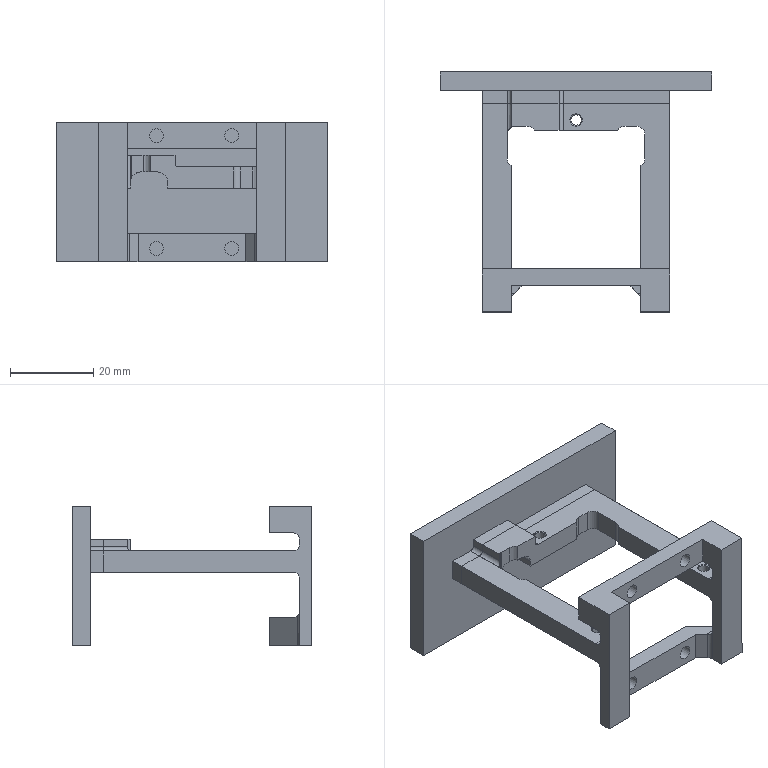NC program | NX | posted with a generic post | part box 65 x 57.5 x 33.5 mm
Whole program, first 1596 of 1898 lines:
N10 G17 G21 G94 G90
(PLANAR_MILL , TOOL : D50面刀)
N12 T01 M6
N14 G53
N16 G17 G0 G90 X52.5 Y-0.5 B0. C0. S3500 M3
N18 G43 Z30.05 H1
N20 Z2.05
N22 G94 G1 Z0.05 F1000.
N24 X25.5
N26 X-25.5
N28 X-52.5
N30 Z2.05
N32 G0 Z30.05
N34 M5
(动态粗 , TOOL : D8-25-D8-60-3T-ROUGH)
N36 T02 M6
N38 G53
N40 G17 G0 G90 X-0.557 Y27.041 B0. C0. S6500 M3
N42 G43 Z30.2 H2
N44 Z-19.5
N46 G94 G1 X-0.555 Y27.016 Z-19.656 F3000.
N48 X-0.553 Y26.991 Z-19.718
N50 X-0.551 Y26.966 Z-19.763
N52 X-0.549 Y26.941 Z-19.8
N54 X-0.548 Y26.916 Z-19.831
N56 X-0.546 Y26.891 Z-19.857
N58 X-0.544 Y26.866 Z-19.88
N60 X-0.542 Y26.841 Z-19.9
N62 X-0.54 Y26.816 Z-19.918
N64 X-0.538 Y26.792 Z-19.933
N66 X-0.536 Y26.767 Z-19.947
N68 X-0.534 Y26.742 Z-19.958
N70 X-0.532 Y26.717 Z-19.968
N72 X-0.53 Y26.692 Z-19.977
N74 X-0.528 Y26.667 Z-19.984
N76 X-0.526 Y26.642 Z-19.99
N78 X-0.525 Y26.617 Z-19.994
N80 X-0.523 Y26.592 Z-19.997
N82 X-0.521 Y26.567 Z-19.999
N84 X-0.519 Y26.542 Z-20.
N86 X-0.415 Y25.2
N88 G3 X0.016 Y24.546 R0.809
N90 X2.614 Y23.818 R7.174
N92 X8.686 Y23.525 R57.315
N94 G1 X23.204 Y23.487
N96 G2 X26.087 Y21.863 R4.371
N98 X27.84 Y18.076 R8.759
N100 X28.414 Y12.488 R30.165
N102 X28.496 Y0.339 R489.81
N104 G1 Y-18.003
N106 G2 X26.977 Y-20.994 R4.21
N108 X23.16 Y-22.822 R8.565
N110 X17.5 Y-23.414 R29.674
N112 X5.276 Y-23.496 R488.293
N114 G1 X-23.021
N116 G2 X-26.01 Y-21.973 R4.208
N118 X-27.81 Y-18.22 R8.513
N120 X-28.405 Y-12.786 R28.448
N122 X-28.496 Y-0.262 R446.293
N124 G1 X-28.495 Y18.022
N126 G2 X-27.03 Y20.961 R4.192
N128 X-23.299 Y22.793 R8.358
N130 X-17.792 Y23.405 R28.015
N132 X-2.672 Y23.477 R466.577
N134 X1.584 Y22.966 R87.011
N136 G3 X10.708 Y22.525 R86.358
N138 G1 X20.58 Y22.488
N140 G2 X24.717 Y20.326 R5.87
N142 X26.404 Y18.298 R4.575
N144 X27.231 Y13.537 R21.682
N146 X27.484 Y4.692 R121.912
N148 G1 X27.495 Y-3.858
N150 X27.485 Y-15.603
N152 G2 X25.908 Y-19.17 R5.72
N154 G1 X25.784 Y-19.369
N156 G2 X23.693 Y-20.871 R5.631
N158 X18.624 Y-22.148 R16.146
N160 X11.284 Y-22.469 R76.065
N162 G1 X1.235 Y-22.496
N164 X-20.471 Y-22.492
N166 G2 X-24.743 Y-20.301 R5.816
N168 X-25.789 Y-19.372 R5.228
N170 X-26.624 Y-17.58 R4.87
N172 X-27.37 Y-11.259 R33.14
N174 X-27.495 Y1.639 R373.69
N176 G1 X-27.496 Y15.322
N178 G2 X-25.942 Y19.135 R5.618
N180 X-24.013 Y20.719 R4.745
N182 X-19.05 Y22.098 R14.951
N184 X-11.938 Y22.462 R64.82
N186 X-3.839 Y22.452 R189.088
N188 X2.452 Y21.889 R227.028
N190 G3 X13.92 Y21.514 R149.911
N192 G2 X18.783 Y21.465 R106.716
N194 X20.893 Y20.966 R8.221
N196 G1 X22.579 Y20.95
N198 G2 X25.558 Y19.628 R4.379
N200 X26.7 Y16.749 R4.363
N202 G1 Y-16.751
N204 X26.595 Y-17.685
N206 X26.284 Y-18.572
N208 X25.784 Y-19.369
N210 X25.119 Y-20.034
N212 X24.322 Y-20.534
N214 X23.435 Y-20.845
N216 G2 X21.599 Y-20.95 R8.97
N218 X7.654 Y-21.481 R161.576
N220 G1 X-1.346 Y-21.495
N222 X-18.92 Y-21.488
N224 G2 X-20.949 Y-20.969 R8.256
N226 G3 X-22.587 Y-20.95 R17.96
N228 G2 X-24.364 Y-20.519 R4.885
N230 G1 X-24.87 Y-20.197
N232 X-24.364 Y-20.519
N234 G3 X-22.587 Y-20.95 R4.887
N236 G1 X21.671
N238 G2 X22.255 Y-22.297 R0.8
N240 X21.801 Y-22.553 Z-19.966 R1.018
N242 G1 X20.825 Y-22.902 Z-19.9
N244 X19.451 Y-23.393 F15000.
N246 X19.318 Y-23.426
N248 X19.182 Y-23.439
N250 X-24.367
N252 G2 X-26.65 Y-22.283 R2.833
N254 G1 X-27.499 Y-21.126
N256 G2 X-27.558 Y-20.265 R0.83
N258 G1 X-26.941 Y-18.827 Z-20. F3000.
N260 X-26.77 Y-18.436
N262 G3 X-26.588 Y-17.726 R1.479
N264 G1 X-26.7 Y-16.782
N266 Y16.751
N268 G2 X-25.557 Y19.63 R4.366
N270 X-22.578 Y20.95 R4.377
N272 G3 X-19.164 Y21.126 R31.383
N274 G2 X-4.473 Y21.421 R151.648
N276 X1.766 Y20.95 R256.713
N278 G1 X21.041
N280 G3 X21.328 Y22.497 R0.8
N282 G1 X19.817 Y22.903 Z-19.9
N284 X19.394 Y23.018 F15000.
N286 X18.967 Y23.121
N288 X18.863 Y23.128
N290 X3.945
N292 G3 X3.408 Y22.921 R0.806
N294 G1 X3.277 Y22.767 Z-19.913 F3000.
N296 X3.174 Y22.593 Z-19.926
N298 X2.596 Y21.588 Z-20.
N300 X2.393 Y21.252
N302 G2 X1.766 Y20.95 R0.802
N304 G1 X-21.634
N306 G2 X-22.431 Y21.626 R0.808
N308 G1 X-22.642 Y22.902
N310 X-22.646 Y22.927 Z-19.999
N312 X-22.65 Y22.951 Z-19.997
N314 X-22.654 Y22.976 Z-19.994
N316 X-22.658 Y23.001 Z-19.99
N318 X-22.662 Y23.025 Z-19.984
N320 X-22.666 Y23.05 Z-19.977
N322 X-22.671 Y23.075 Z-19.968
N324 X-22.675 Y23.099 Z-19.958
N326 X-22.679 Y23.124 Z-19.947
N328 X-22.683 Y23.149 Z-19.933
N330 X-22.687 Y23.173 Z-19.918
N332 X-22.691 Y23.198 Z-19.9
N334 X-22.695 Y23.223 Z-19.88
N336 X-22.699 Y23.247 Z-19.857
N338 X-22.703 Y23.272 Z-19.831
N340 X-22.707 Y23.297 Z-19.8
N342 X-22.711 Y23.321 Z-19.763
N344 X-22.715 Y23.346 Z-19.718
N346 X-22.72 Y23.371 Z-19.656
N348 X-22.724 Y23.395 Z-19.5
N350 G0 Z30.2
N352 X-3.658 Y-3.32
N354 Z0.5
N356 G3 X-3.658 Y-3.32 Z0.105 I-1.698 J3.174
N358 X-3.658 Y-3.32 Z-0.29 I-1.698 J3.174
N360 X-3.658 Y-3.32 Z-0.684 I-1.698 J3.174
N362 X-3.658 Y-3.32 Z-1.079 I-1.698 J3.174
N364 X-3.658 Y-3.32 Z-1.474 I-1.698 J3.174
N366 X-3.658 Y-3.32 Z-1.869 I-1.698 J3.174
N368 X-3.658 Y-3.32 Z-2.264 I-1.698 J3.174
N370 X-3.658 Y-3.32 Z-2.659 I-1.698 J3.174
N372 X-3.658 Y-3.32 Z-3.053 I-1.698 J3.174
N374 X-3.658 Y-3.32 Z-3.448 I-1.698 J3.174
N376 X-3.658 Y-3.32 Z-3.843 I-1.698 J3.174
N378 X-3.658 Y-3.32 Z-4.238 I-1.698 J3.174
N380 X-3.658 Y-3.32 Z-4.633 I-1.698 J3.174
N382 X-3.658 Y-3.32 Z-5.028 I-1.698 J3.174
N384 X-3.658 Y-3.32 Z-5.422 I-1.698 J3.174
N386 X-3.658 Y-3.32 Z-5.817 I-1.698 J3.174
N388 X-3.658 Y-3.32 Z-6.212 I-1.698 J3.174
N390 X-3.658 Y-3.32 Z-6.607 I-1.698 J3.174
N392 X-3.658 Y-3.32 Z-7.002 I-1.698 J3.174
N394 X-3.658 Y-3.32 Z-7.396 I-1.698 J3.174
N396 X-3.658 Y-3.32 Z-7.791 I-1.698 J3.174
N398 X-3.658 Y-3.32 Z-8.186 I-1.698 J3.174
N400 X-3.658 Y-3.32 Z-8.581 I-1.698 J3.174
N402 X-3.658 Y-3.32 Z-8.976 I-1.698 J3.174
N404 X-3.658 Y-3.32 Z-9.371 I-1.698 J3.174
N406 X-3.658 Y-3.32 Z-9.765 I-1.698 J3.174
N408 X-3.658 Y-3.32 Z-10.16 I-1.698 J3.174
N410 X-3.658 Y-3.32 Z-10.555 I-1.698 J3.174
N412 X-3.658 Y-3.32 Z-10.95 I-1.698 J3.174
N414 X-3.658 Y-3.32 Z-11.345 I-1.698 J3.174
N416 X-3.658 Y-3.32 Z-11.74 I-1.698 J3.174
N418 X-3.658 Y-3.32 Z-12.134 I-1.698 J3.174
N420 X-3.658 Y-3.32 Z-12.529 I-1.698 J3.174
N422 X-3.658 Y-3.32 Z-12.924 I-1.698 J3.174
N424 X-3.658 Y-3.32 Z-13.319 I-1.698 J3.174
N426 X-3.658 Y-3.32 Z-13.714 I-1.698 J3.174
N428 X-3.658 Y-3.32 Z-14.108 I-1.698 J3.174
N430 X-3.658 Y-3.32 Z-14.503 I-1.698 J3.174
N432 X-3.658 Y-3.32 Z-14.898 I-1.698 J3.174
N434 X-3.658 Y-3.32 Z-15.293 I-1.698 J3.174
N436 X-3.658 Y-3.32 Z-15.688 I-1.698 J3.174
N438 X-3.658 Y-3.32 Z-16.083 I-1.698 J3.174
N440 X-3.658 Y-3.32 Z-16.477 I-1.698 J3.174
N442 X-3.658 Y-3.32 Z-16.872 I-1.698 J3.174
N444 X-3.658 Y-3.32 Z-17.267 I-1.698 J3.174
N446 X-3.658 Y-3.32 Z-17.662 I-1.698 J3.174
N448 X-3.658 Y-3.32 Z-18.057 I-1.698 J3.174
N450 X-3.658 Y-3.32 Z-18.452 I-1.698 J3.174
N452 X-3.658 Y-3.32 Z-18.846 I-1.698 J3.174
N454 X-3.658 Y-3.32 Z-19.241 I-1.698 J3.174
N456 X-3.658 Y-3.32 Z-19.636 I-1.698 J3.174
N458 X-5.356 Y-3.746 Z-20. R-3.6
N460 X-8.859 Y0.86 R-3.622
N462 X-7.565 Y-3.074 R3.686
N464 X-1.257 Y-0.404 R3.803
N466 X-8.737 Y-2.568 R-4.133
N468 X-0.763 Y0.472 R4.371
N470 X-9.596 Y-2.153 R-4.663
N472 X-0.197 Y0.395 R4.928
N474 X-10.258 Y-2.033 R-5.22
N476 X0.396 Y0.253 R5.501
N478 X-11.072 Y-1.317 R-5.8
N480 X-8.712 Y-5.051 R6.09
N482 X-6.404 Y-6.109 R5.892
N484 X-4.011 Y-6.078 R25.458
N486 X1.014 Y-0.352 R5.969
N488 X-2.88 Y5.767 R6.345
N490 G1 X-3.058 Y5.8
N492 X-7.004 Y5.79
N494 G3 X-10.686 Y3.432 R5.323
N496 X-11.295 Y2.231 R3.646
N498 G1 X-11.287 Y-1.937
N500 G3 X-9.152 Y-5.489 R5.512
N502 X-8.184 Y-6.084 R3.454
N504 X-6.386 Y-6.109 R15.894
N506 G1 X-8.261 Y-6.105
N508 G2 X-10.345 Y-4.765 R3.942
N510 X-11.289 Y-3.176 R4.436
N512 G1 X-11.3 Y-1.745
N514 X-11.285 Y-3.669
N516 G3 X-9.606 Y-6.046 R3.591
N518 G1 X-9.335 Y-6.109
N520 X-8.135
N522 X-9.56 Y-6.104
N524 G2 X-11.28 Y-4.463 R2.722
N526 X-11.3 Y-3.507 R14.66
N528 G1 X-11.283 Y-4.769
N530 G3 X-10.436 Y-6.026 R1.868
N532 G1 X-10.128 Y-6.109
N534 X-9.453
N536 G2 X-10.452 Y-6.069 R3.999
N538 X-11.3 Y-5.07 R1.309
N540 G1 Y-4.62
N542 G3 X-11.26 Y-5.459 R3.698
N544 X-10.162 Y-6.109 R0.982
N546 G1 X-2.885 Y-6.096
N548 G3 X0.214 Y-4.217 R4.93
N550 X-1.467 Y5.723 R6.84
N552 G1 X-1.76 Y5.8
N554 X-3.11
N556 X-1.61
N558 G2 X0.114 Y4.765 R3.423
N560 X-0.224 Y-5.193 R6.955
N562 X-1.699 Y-6.091 R4.625
N564 X-3.096 Y-6.109 R24.229
N566 G3 X-1.183 Y-6.077 R16.279
N568 X1.17 Y-4.492 R4.334
N570 X0.54 Y5.228 R7.352
N572 X-0.308 Y5.785 R1.994
N574 G1 X-1.685 Y5.8
N576 X-0.185 Y5.794
N578 G2 X1.544 Y4.545 R3.475
N580 X1.363 Y-4.834 R7.503
N582 X-0.323 Y-6.086 R4.306
N584 X-1.521 Y-6.109 R8.553
N586 G3 X0.057 Y-6.087 R16.365
N588 X2.198 Y-4.634 R3.913
N590 X3.49 Y2.138 R7.698
N592 X1.312 Y5.621 R6.406
N594 X0.833 Y5.8 R1.065
N596 G1 X-0.292
N598 X1.057 Y5.795
N600 G2 X2.618 Y4.671 R3.155
N602 X4.144 Y-0.576 R7.5
N604 X2.037 Y-5.335 R7.228
N606 X0.86 Y-6.094 R3.079
N608 G1 X-0.143 Y-6.109
N610 G3 X1.339 Y-6.066 R8.535
N612 X3.42 Y-4.506 R4.035
N614 X4.562 Y2.281 R8.024
N616 X2.594 Y5.553 R6.327
N618 X2.032 Y5.8 R1.021
N620 G1 X0.982
N622 X2.257 Y5.794
N624 G2 X3.81 Y4.624 R3.109
N626 X5.241 Y-0.438 R7.624
N628 X3.293 Y-5.214 R7.44
N630 X2.051 Y-6.083 R3.529
N632 X1.004 Y-6.109 R5.719
N634 G3 X2.35 Y-6.091 R35.512
N636 X4.329 Y-4.758 R3.592
N638 X5.926 Y0.73 R7.853
N640 X4.199 Y5.131 R7.317
N642 X3.328 Y5.779 R1.966
N644 X2.14 Y5.8 R11.657
N646 G1 X3.414 Y5.795
N648 G2 X4.878 Y4.712 R2.954
N650 X6.352 Y0.036 R7.493
N652 X4.55 Y-5.06 R7.745
N654 X3.176 Y-6.084 R3.544
N656 X2.203 Y-6.109 R5.878
N658 G3 X3.483 Y-6.088 R17.141
N660 X5.459 Y-4.722 R3.575
N662 X7.029 Y0.74 R7.949
N664 X5.422 Y5.035 R7.397
N666 X4.527 Y5.764 R2.287
N668 X3.289 Y5.8 R6.426
N670 G1 X4.563 Y5.794
N672 G2 X6.084 Y4.615 R3.027
N674 X7.451 Y-0.121 R7.618
N676 X5.659 Y-5.055 R7.762
N678 X4.323 Y-6.073 R3.885
N680 X3.309 Y-6.109 R4.91
N682 G3 X4.587 Y-6.089 R20.116
N684 X6.558 Y-4.725 R3.565
N686 X8.138 Y0.69 R7.989
N688 X6.578 Y5.003 R7.442
N690 X5.695 Y5.754 R2.464
N692 G1 X5.475 Y5.8
N694 X4.425
N696 X5.625
N698 G2 X6.94 Y4.94 R2.475
N700 X8.514 Y1.023 R6.976
N702 X7.035 Y-4.724 R8.249
N704 X5.401 Y-6.08 R3.963
N706 X4.417 Y-6.109 R4.438
N708 G1 X5.668 Y-6.094
N710 G3 X7.529 Y-4.886 R3.434
N712 X9.257 Y0.013 R7.786
N714 X7.835 Y4.833 R7.755
N716 X6.847 Y5.743 R2.918
N718 G1 X6.597 Y5.8
N720 X5.622
N722 X6.747
N724 G2 X8.063 Y4.936 R2.474
N726 X9.632 Y0.922 R7.01
N728 X8.109 Y-4.76 R8.227
N730 X6.55 Y-6.068 R4.257
N732 X5.513 Y-6.109 R4.583
N734 G1 X6.782 Y-6.091
N736 G3 X8.668 Y-4.838 R3.448
N738 X10.365 Y0.118 R7.857
N740 X8.918 Y4.877 R7.69
N742 X8.005 Y5.727 R3.189
N744 G1 X7.715 Y5.8
N746 X6.74
N748 X7.865
N750 G2 X9.167 Y4.95 R2.457
N752 X10.732 Y0.977 R6.956
N754 X9.148 Y-4.84 R8.209
N756 X7.667 Y-6.063 R4.243
N758 X6.622 Y-6.109 R4.195
N760 G3 X7.895 Y-6.09 R28.393
N762 X9.864 Y-4.726 R3.566
N764 X11.3 Y-1.485 R7.324
N766 X11.273 Y1.564 R49.051
N768 X9.521 Y5.421 R6.195
N770 X8.817 Y5.8 R1.157
N772 G1 X7.842
N774 X9.042 Y5.794
N776 G2 X10.557 Y4.573 R2.98
N778 X11.3 Y3.024 R4.23
N780 G1 Y1.149
N782 X11.285 Y3.699
N784 G3 X10.104 Y5.693 R3.046
N786 X9.747 Y5.8 R2.866
N788 G1 X8.922
N790 X9.897
N792 G2 X11.111 Y4.838 R1.973
N794 X11.3 Y4.338 R1.246
N796 G1 Y3.513
N798 G3 X11.279 Y4.776 R13.612
N800 X10.572 Y5.743 R1.302
N802 X9.874 Y5.8 R1.848
N804 G2 X10.72 Y5.733 R2.207
N806 X11.3 Y4.587 R1.09
N808 G3 X11.097 Y5.47 R1.263
N810 X10.678 Y5.749 R1.014
N812 G2 X11.271 Y5.11 R0.873
N814 G1 X11.3 Y4.887
N816 X11.287 Y-2.268
N818 G2 X8.862 Y-6.017 R5.053
N820 G1 X8.531 Y-6.109
N822 X7.706
N824 X8.961 Y-6.093
N826 G3 X10.866 Y-4.758 R3.351
N828 X11.3 Y-3.911 R1.768
N830 G1 Y-2.036
N832 Y-4.061
N834 G2 X9.646 Y-6.085 R2.734
N836 X8.823 Y-6.109 R6.586
N838 G3 X9.953 Y-6.085 R8.9
N840 X11.238 Y-5.122 R1.964
N842 G1 X11.3 Y-4.856
N844 Y-4.031
N846 Y-5.006
N848 G2 X10.21 Y-6.109 R1.37
N850 G1 X9.76
N852 G3 X10.65 Y-6.069 R3.988
N854 X11.3 Y-4.971 R0.982
N856 X10.857 Y-4.207 R0.881
N858 G1 X10.699 Y-4.117
N860 X9.341 Y-3.34 Z-19.9
N862 X-3.211 Y3.834 F15000.
N864 X-4.569 Y4.611 Z-20. F3000.
N866 X-6.446 Y5.684
N868 G3 X-6.883 Y5.8 R0.9
N870 X-8.373 Y5.744 R7.486
N872 X-11.235 Y3.628 R4.771
N874 G1 X-11.3 Y3.35
N876 Y2.15
N878 Y3.5
N880 G2 X-10.238 Y5.121 R2.944
N882 X-9.087 Y5.791 R2.934
N884 G1 X-7.962 Y5.8
N886 X-9.514 Y5.784
N888 G3 X-11.21 Y4.655 R2.676
N890 G1 X-11.3 Y4.328
N892 Y3.428
N894 Y4.478
N896 G2 X-10.03 Y5.794 R1.78
N898 G1 X-9.376 Y5.8
N900 G3 X-10.412 Y5.774 R6.347
N902 X-11.287 Y4.967 R1.112
N904 G1 X-11.3 Y4.427
N906 G2 X-11.179 Y5.344 R1.826
N908 X-10.237 Y5.8 R0.951
N910 G3 X-10.818 Y5.695 R1.166
N912 X-11.222 Y5.248 R0.862
N914 X-10.68 Y4.179 R0.808
N916 G1 X-9.337 Y3.813
N918 X-9.313 Y3.806 Z-19.999
N920 X-9.289 Y3.8 Z-19.997
N922 X-9.264 Y3.793 Z-19.994
N924 X-9.24 Y3.786 Z-19.99
N926 X-9.216 Y3.78 Z-19.984
N928 X-9.192 Y3.773 Z-19.977
N930 X-9.168 Y3.767 Z-19.968
N932 X-9.144 Y3.76 Z-19.958
N934 X-9.12 Y3.754 Z-19.947
N936 X-9.096 Y3.747 Z-19.933
N938 X-9.071 Y3.74 Z-19.918
N940 X-9.047 Y3.734 Z-19.9
N942 X-9.023 Y3.727 Z-19.88
N944 X-8.999 Y3.721 Z-19.857
N946 X-8.975 Y3.714 Z-19.831
N948 X-8.951 Y3.708 Z-19.8
N950 X-8.927 Y3.701 Z-19.763
N952 X-8.903 Y3.694 Z-19.718
N954 X-8.879 Y3.688 Z-19.656
N956 X-8.854 Y3.681 Z-19.5
N958 G0 Z30.2
N960 X-13.615 Y23.401
N962 Z-5.7
N964 G1 X-13.612 Y23.376 Z-5.856
N966 X-13.608 Y23.352 Z-5.918
N968 X-13.605 Y23.327 Z-5.964
N970 X-13.602 Y23.302 Z-6.
N972 X-13.598 Y23.277 Z-6.031
N974 X-13.595 Y23.252 Z-6.057
N976 X-13.591 Y23.228 Z-6.08
N978 X-13.588 Y23.203 Z-6.1
N980 X-13.585 Y23.178 Z-6.118
N982 X-13.581 Y23.153 Z-6.133
N984 X-13.578 Y23.129 Z-6.147
N986 X-13.574 Y23.104 Z-6.158
N988 X-13.571 Y23.079 Z-6.168
N990 X-13.568 Y23.054 Z-6.177
N992 X-13.564 Y23.03 Z-6.184
N994 X-13.561 Y23.005 Z-6.19
N996 X-13.557 Y22.98 Z-6.194
N998 X-13.554 Y22.955 Z-6.198
N1000 X-13.55 Y22.93 Z-6.199
N1002 X-13.547 Y22.906 Z-6.2
N1004 X-13.368 Y21.604
N1006 G3 X-12.654 Y20.91 R0.808
N1008 G1 X-12.082 Y20.849
N1010 G3 X-8.705 Y20.163 R11.109
N1012 X-1.005 Y19.957 R110.469
N1014 G1 X10.087 Y19.953
N1016 X10.39 Y20.045
N1018 X11.188 Y20.541
N1020 X12.082 Y20.849
N1022 X12.678 Y20.913
N1024 X12.082 Y20.849
N1026 X11.188 Y20.541
N1028 G2 X10.151 Y19.916 R9.659
N1030 X7.314 Y19.475 R10.662
N1032 X-3.84 Y19.387 R192.319
N1034 X-9.65 Y19.731 R45.951
N1036 X-10.386 Y20.042 R1.126
N1038 G3 X-11.259 Y20.565 R36.07
N1040 G2 X-10.31 Y19.968 R5.604
N1042 G3 X-8.885 Y19.171 R3.052
N1044 X-4.648 Y18.528 R18.337
N1046 X6.951 Y18.511 R109.452
N1048 X9.24 Y18.878 R10.047
N1050 X9.714 Y19.377 R1.13
N1052 G1 X10.386 Y20.042
N1054 X9.714 Y19.377
N1056 G2 X8.809 Y18.585 R1.478
N1058 X5.568 Y17.954 R11.199
N1060 X-5.804 Y18.066 R74.975
N1062 X-9.21 Y18.841 R11.936
N1064 X-9.714 Y19.377 R1.174
N1066 G1 X-10.14 Y19.799
N1068 G2 X-9.392 Y18.87 R3.109
N1070 G3 X-7.597 Y17.793 R4.089
N1072 X-3.244 Y17.016 R17.771
N1074 X5.796 Y17.063 R52.282
N1076 X8.732 Y17.815 R8.817
N1078 X9.207 Y18.579 R1.274
N1080 G1 X9.529 Y19.086
N1082 G3 X9.024 Y18.064 R2.816
N1084 G2 X8.082 Y17.31 R2.072
N1086 X4.654 Y16.484 R10.658
N1088 X-5.322 Y16.723 R41.444
N1090 X-8.53 Y17.761 R9.708
N1092 X-9.207 Y18.579 R1.195
N1094 G1 X-9.408 Y18.896
N1096 G2 X-9.033 Y18.088 R2.481
N1098 G3 X-7.659 Y16.842 R3.111
N1100 X-3.706 Y15.697 R12.047
N1102 X5.307 Y15.686 R32.782
N1104 X8.359 Y16.714 R8.073
N1106 X8.891 Y17.689 R1.081
N1108 G1 X9.067 Y18.183
N1110 G3 X8.834 Y17.209 R2.524
N1112 G2 X8.034 Y16.292 R1.818
N1114 X4.861 Y15.177 R8.286
N1116 X-5.073 Y15.428 R28.131
N1118 X-8.232 Y16.751 R8.571
N1120 X-8.858 Y17.485 R1.501
N1122 G3 X-9.041 Y18.113 R2.699
N1124 G2 X-8.849 Y17.335 R2.106
N1126 G3 X-7.842 Y16.004 R2.568
N1128 X-4.331 Y14.514 R9.107
N1130 X5.189 Y14.387 R23.99
N1132 X8.189 Y15.629 R7.632
N1134 X8.78 Y16.488 R1.23
N1136 G2 X8.85 Y17.347 R7.238
N1138 G3 X8.774 Y16.263 R7.612
N1140 G2 X7.766 Y15.057 R2.443
N1142 X4.428 Y13.798 R8.7
N1144 X-5.093 Y14.209 R21.894
N1146 X-8.217 Y15.853 R7.677
N1148 X-8.78 Y16.713 R1.624
N1150 G1 X-8.85 Y17.345
N1152 X-8.755 Y16.35
N1154 G3 X-7.539 Y14.744 R3.252
N1156 X-4.273 Y13.28 R7.788
N1158 X5.422 Y13.194 R18.849
N1160 X8.307 Y14.688 R7.014
N1162 X8.78 Y15.473 R1.249
N1164 G1 Y16.373
N1166 Y15.323
N1168 G2 X7.888 Y14.042 R2.375
N1170 G1 X7.139 Y13.485
N1172 G3 X6.624 Y11.079 R2.764
N1174 X8.469 Y8.225 R5.262
N1176 X10.067 Y7.003 R67.019
N1178 X10.776 Y6.376 R14.395
N1180 G2 X11.3 Y5.517 R1.435
N1182 G1 Y5.142
N1184 G3 X11.125 Y6.117 R1.636
N1186 X10.183 Y6.875 R4.64
N1188 G2 X8.874 Y9.125 R4.537
N1190 G1 X8.78 Y10.001
N1192 Y15.326
N1194 G3 X8.366 Y16.072 R0.881
N1196 X7.814 Y16.215 Z-6.163 R1.09
N1198 G1 X6.829 Y16.287 Z-6.1
N1200 X-6.87 Y17.294 F15000.
N1202 X-7.412 Y17.338 Z-6.135 F3000.
N1204 X-7.955 Y17.366 Z-6.17
N1206 G3 X-8.4 Y17.212 Z-6.2 R0.917
N1208 X-8.78 Y16.488 R0.881
N1210 X-8.125 Y14.722 R2.388
N1212 X-6.701 Y13.517 R6.523
N1214 G2 X-6.229 Y11.901 R2.24
N1216 X-7.506 Y9.352 R3.792
N1218 X-9.278 Y7.97 R14.227
N1220 G3 X-9.591 Y7.527 R1.783
N1222 G2 X-10.843 Y6.4 R4.753
N1224 G3 X-11.3 Y5.554 R1.057
N1226 G1 Y5.179
N1228 X-11.292 Y5.668
N1230 G2 X-10.948 Y6.312 R1.006
N1232 G1 X-10.183 Y6.875
N1234 X-9.591 Y7.527
N1236 G3 X-8.835 Y8.806 R23.849
N1238 X-8.536 Y12.34 R6.037
N1240 G1 X-8.78 Y13.522
N1242 Y16.147
N1244 Y9.999
N1246 G2 X-9.149 Y8.288 R4.873
N1248 G1 X-9.337 Y7.964
N1250 G3 X-9.214 Y6.99 R0.808
N1252 G1 X-8.289 Y6.052
N1254 X-8.272 Y6.034 Z-6.199
N1256 X-8.254 Y6.016 Z-6.198
N1258 X-8.236 Y5.998 Z-6.194
N1260 X-8.219 Y5.981 Z-6.19
N1262 X-8.201 Y5.963 Z-6.184
N1264 X-8.184 Y5.945 Z-6.177
N1266 X-8.166 Y5.927 Z-6.168
N1268 X-8.149 Y5.909 Z-6.158
N1270 X-8.131 Y5.892 Z-6.147
N1272 X-8.114 Y5.874 Z-6.133
N1274 X-8.096 Y5.856 Z-6.118
N1276 X-8.078 Y5.838 Z-6.1
N1278 X-8.061 Y5.82 Z-6.08
N1280 X-8.043 Y5.803 Z-6.057
N1282 X-8.026 Y5.785 Z-6.031
N1284 X-8.008 Y5.767 Z-6.
N1286 X-7.991 Y5.749 Z-5.964
N1288 X-7.973 Y5.731 Z-5.918
N1290 X-7.956 Y5.714 Z-5.856
N1292 X-7.938 Y5.696 Z-5.7
N1294 G0 Z30.2
N1296 X-13.137 Y23.389
N1298 Z-5.5
N1300 G1 X-13.132 Y23.364 Z-5.656
N1302 X-13.128 Y23.34 Z-5.718
N1304 X-13.124 Y23.315 Z-5.763
N1306 X-13.119 Y23.29 Z-5.8
N1308 X-13.115 Y23.266 Z-5.831
N1310 X-13.111 Y23.241 Z-5.857
N1312 X-13.106 Y23.216 Z-5.88
N1314 X-13.102 Y23.192 Z-5.9
N1316 X-13.097 Y23.167 Z-5.918
N1318 X-13.093 Y23.143 Z-5.933
N1320 X-13.089 Y23.118 Z-5.947
N1322 X-13.084 Y23.093 Z-5.958
N1324 X-13.08 Y23.069 Z-5.968
N1326 X-13.076 Y23.044 Z-5.977
N1328 X-13.071 Y23.02 Z-5.984
N1330 X-13.067 Y22.995 Z-5.99
N1332 X-13.062 Y22.97 Z-5.994
N1334 X-13.058 Y22.946 Z-5.997
N1336 X-13.054 Y22.921 Z-5.999
N1338 X-13.049 Y22.897 Z-6.
N1340 X-12.794 Y21.462
N1342 G3 X-12.264 Y20.84 R0.809
N1344 G1 X-11.385 Y20.534
N1346 X-10.584 Y20.035
N1348 X-9.914 Y19.371
N1350 X-9.406 Y18.575
N1352 X-9.087 Y17.687
N1354 X-8.973 Y16.749
N1356 Y9.999
N1358 G2 X-9.721 Y7.62 R4.534
N1360 X-10.879 Y6.5 R4.764
N1362 G3 X-11.232 Y6.018 R1.139
N1364 X-10.362 Y4.921 R0.808
N1366 G1 X-9.338 Y5.073
N1368 X-9.313 Y5.077 Z-5.999
N1370 X-9.288 Y5.081 Z-5.997
N1372 X-9.264 Y5.084 Z-5.994
N1374 X-9.239 Y5.088 Z-5.99
N1376 X-9.214 Y5.092 Z-5.984
N1378 X-9.189 Y5.095 Z-5.977
N1380 X-9.165 Y5.099 Z-5.968
N1382 X-9.14 Y5.103 Z-5.958
N1384 X-9.115 Y5.106 Z-5.947
N1386 X-9.09 Y5.11 Z-5.933
N1388 X-9.066 Y5.114 Z-5.918
N1390 X-9.041 Y5.117 Z-5.9
N1392 X-9.016 Y5.121 Z-5.88
N1394 X-8.992 Y5.125 Z-5.857
N1396 X-8.967 Y5.128 Z-5.831
N1398 X-8.942 Y5.132 Z-5.8
N1400 X-8.917 Y5.136 Z-5.763
N1402 X-8.893 Y5.139 Z-5.718
N1404 X-8.868 Y5.143 Z-5.656
N1406 X-8.843 Y5.147 Z-5.5
N1408 G0 Z30.2
N1410 X-14.832 Y23.401
N1412 Z-4.5
N1414 G1 X-14.828 Y23.376 Z-4.656
N1416 X-14.824 Y23.351 Z-4.718
N1418 X-14.821 Y23.326 Z-4.763
N1420 X-14.817 Y23.302 Z-4.8
N1422 X-14.814 Y23.277 Z-4.831
N1424 X-14.81 Y23.252 Z-4.857
N1426 X-14.807 Y23.227 Z-4.88
N1428 X-14.803 Y23.203 Z-4.9
N1430 X-14.8 Y23.178 Z-4.918
N1432 X-14.796 Y23.153 Z-4.933
N1434 X-14.793 Y23.128 Z-4.947
N1436 X-14.789 Y23.104 Z-4.958
N1438 X-14.785 Y23.079 Z-4.968
N1440 X-14.782 Y23.054 Z-4.977
N1442 X-14.778 Y23.029 Z-4.984
N1444 X-14.775 Y23.005 Z-4.99
N1446 X-14.771 Y22.98 Z-4.994
N1448 X-14.768 Y22.955 Z-4.997
N1450 X-14.764 Y22.93 Z-4.999
N1452 X-14.761 Y22.906 Z-5.
N1454 X-14.573 Y21.598
N1456 G3 X-13.866 Y20.91 R0.808
N1458 G1 X-13.278 Y20.842
N1460 X-12.388 Y20.53
N1462 X-11.589 Y20.03
N1464 X-10.919 Y19.367
N1466 X-10.411 Y18.572
N1468 X-10.09 Y17.685
N1470 X-9.973 Y16.749
N1472 Y9.999
N1474 G2 X-11.064 Y7.19 R4.338
N1476 G3 X-11.3 Y6.536 R1.111
N1478 G1 Y5.936
N1480 G3 X-10.496 Y5.128 R0.808
N1482 G1 X-9.331 Y5.122
N1484 X-9.306 Z-4.999
N1486 X-9.281 Z-4.997
N1488 X-9.256 Z-4.994
N1490 X-9.231 Z-4.99
N1492 X-9.206 Z-4.984
N1494 X-9.181 Z-4.977
N1496 X-9.156 Z-4.968
N1498 X-9.131 Z-4.958
N1500 X-9.106 Y5.121 Z-4.947
N1502 X-9.081 Z-4.933
N1504 X-9.056 Z-4.918
N1506 X-9.031 Z-4.9
N1508 X-9.006 Z-4.88
N1510 X-8.981 Z-4.857
N1512 X-8.956 Z-4.831
N1514 X-8.931 Z-4.8
N1516 X-8.906 Z-4.763
N1518 X-8.881 Y5.12 Z-4.718
N1520 X-8.856 Z-4.656
N1522 X-8.831 Z-4.5
N1524 G0 Z30.2
N1526 X-15.783 Y23.401
N1528 Z-3.5
N1530 G1 X-15.78 Y23.376 Z-3.656
N1532 X-15.776 Y23.352 Z-3.718
N1534 X-15.773 Y23.327 Z-3.763
N1536 X-15.77 Y23.302 Z-3.8
N1538 X-15.766 Y23.277 Z-3.831
N1540 X-15.763 Y23.252 Z-3.857
N1542 X-15.759 Y23.228 Z-3.88
N1544 X-15.756 Y23.203 Z-3.9
N1546 X-15.752 Y23.178 Z-3.918
N1548 X-15.749 Y23.153 Z-3.933
N1550 X-15.746 Y23.129 Z-3.947
N1552 X-15.742 Y23.104 Z-3.958
N1554 X-15.739 Y23.079 Z-3.968
N1556 X-15.735 Y23.054 Z-3.977
N1558 X-15.732 Y23.03 Z-3.984
N1560 X-15.729 Y23.005 Z-3.99
N1562 X-15.725 Y22.98 Z-3.994
N1564 X-15.722 Y22.955 Z-3.997
N1566 X-15.718 Y22.93 Z-3.999
N1568 X-15.715 Y22.906 Z-4.
N1570 X-15.535 Y21.603
N1572 G3 X-14.824 Y20.91 R0.808
N1574 G1 X-14.244 Y20.846
N1576 X-13.354 Y20.536
N1578 X-12.556 Y20.036
N1580 X-11.888 Y19.371
N1582 X-11.386 Y18.575
N1584 X-11.073 Y17.686
N1586 X-10.966 Y16.749
N1588 Y9.938
N1590 G2 X-11.283 Y8.273 R5.42
N1592 G1 X-11.3 Y6.744
N1594 G3 X-10.366 Y5.946 R0.808
N1596 G1 X-9.341 Y6.108
N1598 X-9.316 Y6.112 Z-3.999
N1600 X-9.291 Y6.115 Z-3.997
N1602 X-9.266 Y6.119 Z-3.994
N1604 X-9.242 Y6.123 Z-3.99
N1606 X-9.217 Y6.127 Z-3.984
N1608 X-9.192 Y6.131 Z-3.977
N1610 X-9.168 Y6.135 Z-3.968
N1612 X-9.143 Y6.139 Z-3.958
N1614 X-9.118 Y6.143 Z-3.947
N1616 X-9.094 Y6.147 Z-3.933
N1618 X-9.069 Y6.151 Z-3.918
N1620 X-9.044 Y6.154 Z-3.9
N1622 X-9.02 Y6.158 Z-3.88
N1624 X-8.995 Y6.162 Z-3.857
N1626 X-8.97 Y6.166 Z-3.831
N1628 X-8.945 Y6.17 Z-3.8
N1630 X-8.921 Y6.174 Z-3.763
N1632 X-8.896 Y6.178 Z-3.718
N1634 X-8.871 Y6.182 Z-3.656
N1636 X-8.847 Y6.186 Z-3.5
N1638 G0 Z30.2
N1640 X-15.883 Y23.403
N1642 Z-2.5
N1644 G1 X-15.88 Y23.378 Z-2.656
N1646 X-15.878 Y23.353 Z-2.718
N1648 X-15.875 Y23.328 Z-2.763
N1650 X-15.872 Y23.303 Z-2.8
N1652 X-15.869 Y23.279 Z-2.831
N1654 X-15.867 Y23.254 Z-2.857
N1656 X-15.864 Y23.229 Z-2.88
N1658 X-15.861 Y23.204 Z-2.9
N1660 X-15.859 Y23.179 Z-2.918
N1662 X-15.856 Y23.154 Z-2.933
N1664 X-15.853 Y23.129 Z-2.947
N1666 X-15.851 Y23.105 Z-2.958
N1668 X-15.848 Y23.08 Z-2.968
N1670 X-15.845 Y23.055 Z-2.977
N1672 X-15.843 Y23.03 Z-2.984
N1674 X-15.84 Y23.005 Z-2.99
N1676 X-15.837 Y22.98 Z-2.994
N1678 X-15.834 Y22.955 Z-2.997
N1680 X-15.832 Y22.931 Z-2.999
N1682 X-15.829 Y22.906 Z-3.
N1684 X-15.689 Y21.614
N1686 G3 X-14.966 Y20.897 R0.808
N1688 G1 X-14.653 Y20.866
N1690 X-13.842 Y20.609
N1692 X-13.022 Y20.141
N1694 X-12.328 Y19.503
N1696 X-11.794 Y18.725
N1698 G2 X-11.331 Y17.295 R5.639
N1700 G1 X-11.3 Y16.736
N1702 Y8.261
N1704 G3 X-10.601 Y7.46 R0.808
N1706 G1 X-9.344 Y7.288
N1708 X-9.319 Y7.285 Z-2.999
N1710 X-9.295 Y7.282 Z-2.997
N1712 X-9.27 Y7.278 Z-2.994
N1714 X-9.245 Y7.275 Z-2.99
N1716 X-9.22 Y7.272 Z-2.984
N1718 X-9.196 Y7.268 Z-2.977
N1720 X-9.171 Y7.265 Z-2.968
N1722 X-9.146 Y7.261 Z-2.958
N1724 X-9.121 Y7.258 Z-2.947
N1726 X-9.097 Y7.255 Z-2.933
N1728 X-9.072 Y7.251 Z-2.918
N1730 X-9.047 Y7.248 Z-2.9
N1732 X-9.022 Y7.244 Z-2.88
N1734 X-8.997 Y7.241 Z-2.857
N1736 X-8.973 Y7.238 Z-2.831
N1738 X-8.948 Y7.234 Z-2.8
N1740 X-8.923 Y7.231 Z-2.763
N1742 X-8.898 Y7.228 Z-2.718
N1744 X-8.874 Y7.224 Z-2.656
N1746 X-8.849 Y7.221 Z-2.5
N1748 G0 Z30.2
N1750 X8.849 Y4.682
N1752 Z-5.5
N1754 G1 X8.874 Y4.685 Z-5.656
N1756 X8.899 Y4.689 Z-5.718
N1758 X8.923 Y4.692 Z-5.763
N1760 X8.948 Y4.696 Z-5.8
N1762 X8.973 Y4.699 Z-5.831
N1764 X8.998 Y4.703 Z-5.857
N1766 X9.022 Y4.707 Z-5.88
N1768 X9.047 Y4.71 Z-5.9
N1770 X9.072 Y4.714 Z-5.918
N1772 X9.097 Y4.717 Z-5.933
N1774 X9.121 Y4.721 Z-5.947
N1776 X9.146 Y4.724 Z-5.958
N1778 X9.171 Y4.728 Z-5.968
N1780 X9.196 Y4.731 Z-5.977
N1782 X9.22 Y4.735 Z-5.984
N1784 X9.245 Y4.738 Z-5.99
N1786 X9.27 Y4.742 Z-5.994
N1788 X9.295 Y4.745 Z-5.997
N1790 X9.319 Y4.749 Z-5.999
N1792 X9.344 Y4.753 Z-6.
N1794 X10.591 Y4.931
N1796 G3 X11.227 Y6.029 R0.808
N1798 X10.877 Y6.5 R1.156
N1800 G2 X9.313 Y8.36 R4.477
N1802 X8.973 Y10.001 R4.892
N1804 G1 Y16.751
N1806 X9.093 Y17.708
N1808 X9.426 Y18.614
N1810 X9.955 Y19.422
N1812 X10.652 Y20.089
N1814 X11.483 Y20.581
N1816 X12.34 Y20.854
N1818 G3 X12.891 Y21.481 R0.809
N1820 G1 X13.146 Y22.894
N1822 X13.15 Y22.918 Z-5.999
N1824 X13.154 Y22.943 Z-5.997
N1826 X13.159 Y22.968 Z-5.994
N1828 X13.163 Y22.992 Z-5.99
N1830 X13.168 Y23.017 Z-5.984
N1832 X13.172 Y23.041 Z-5.977
N1834 X13.177 Y23.066 Z-5.968
N1836 X13.181 Y23.091 Z-5.958
N1838 X13.185 Y23.115 Z-5.947
N1840 X13.19 Y23.14 Z-5.933
N1842 X13.194 Y23.164 Z-5.918
N1844 X13.199 Y23.189 Z-5.9
N1846 X13.203 Y23.214 Z-5.88
N1848 X13.208 Y23.238 Z-5.857
N1850 X13.212 Y23.263 Z-5.831
N1852 X13.216 Y23.287 Z-5.8
N1854 X13.221 Y23.312 Z-5.763
N1856 X13.225 Y23.337 Z-5.718
N1858 X13.23 Y23.361 Z-5.656
N1860 X13.234 Y23.386 Z-5.5
N1862 G0 Z30.2
N1864 X8.844 Y5.148
N1866 Z-4.5
N1868 G1 X8.869 Z-4.656
N1870 X8.894 Z-4.718
N1872 X8.919 Y5.149 Z-4.763
N1874 X8.944 Z-4.8
N1876 X8.969 Z-4.831
N1878 X8.994 Y5.15 Z-4.857
N1880 X9.019 Z-4.88
N1882 X9.044 Z-4.9
N1884 X9.069 Y5.151 Z-4.918
N1886 X9.094 Z-4.933
N1888 X9.119 Z-4.947
N1890 X9.144 Y5.152 Z-4.958
N1892 X9.169 Z-4.968
N1894 X9.194 Z-4.977
N1896 X9.219 Y5.153 Z-4.984
N1898 X9.244 Z-4.99
N1900 X9.269 Z-4.994
N1902 X9.294 Y5.154 Z-4.997
N1904 X9.319 Z-4.999
N1906 X9.344 Z-5.
N1908 X10.503 Y5.17
N1910 G3 X11.3 Y5.97 R0.808
N1912 X11.031 Y6.805 R2.959
N1914 X10.731 Y7.626 R6.4
N1916 G2 X9.973 Y10.001 R4.292
N1918 G1 Y16.751
N1920 X10.083 Y17.689
N1922 X10.4 Y18.579
N1924 X10.907 Y19.377
N1926 X11.578 Y20.042
N1928 X12.381 Y20.541
N1930 X13.274 Y20.848
N1932 X13.871 Y20.913
N1934 X13.274 Y20.848
N1936 X12.381 Y20.541
N1938 X11.578 Y20.042
N1940 X10.907 Y19.377
N1942 X10.4 Y18.579
N1944 X10.083 Y17.689
N1946 X9.973 Y16.751
N1948 Y10.001
N1950 G3 X11.063 Y7.191 R4.338
N1952 G2 X11.3 Y6.538 R1.109
N1954 G1 Y5.938
N1956 G2 X10.496 Y5.13 R0.808
N1958 G1 X9.344 Y5.124
N1960 X9.319 Z-4.999
N1962 X9.294 Y5.123 Z-4.997
N1964 X9.269 Z-4.994
N1966 X9.244 Z-4.99
N1968 X9.219 Z-4.984
N1970 X9.194 Z-4.977
N1972 X9.169 Z-4.968
N1974 X9.144 Z-4.958
N1976 X9.119 Y5.122 Z-4.947
N1978 X9.094 Z-4.933
N1980 X9.069 Z-4.918
N1982 X9.044 Z-4.9
N1984 X9.019 Z-4.88
N1986 X8.994 Z-4.857
N1988 X8.969 Z-4.831
N1990 X8.944 Y5.121 Z-4.8
N1992 X8.919 Z-4.763
N1994 X8.894 Z-4.718
N1996 X8.869 Z-4.656
N1998 X8.844 Z-4.5
N2000 G0 Z30.2
N2002 X8.83 Y6.278
N2004 Z-3.5
N2006 G1 X8.855 Y6.275 Z-3.656
N2008 X8.88 Y6.271 Z-3.718
N2010 X8.904 Y6.267 Z-3.763
N2012 X8.929 Y6.263 Z-3.8
N2014 X8.954 Y6.259 Z-3.831
N2016 X8.978 Y6.255 Z-3.857
N2018 X9.003 Y6.251 Z-3.88
N2020 X9.028 Y6.247 Z-3.9
N2022 X9.052 Y6.243 Z-3.918
N2024 X9.077 Y6.239 Z-3.933
N2026 X9.102 Y6.235 Z-3.947
N2028 X9.126 Y6.231 Z-3.958
N2030 X9.151 Y6.227 Z-3.968
N2032 X9.176 Y6.223 Z-3.977
N2034 X9.2 Y6.219 Z-3.984
N2036 X9.225 Y6.215 Z-3.99
N2038 X9.25 Y6.211 Z-3.994
N2040 X9.275 Y6.207 Z-3.997
N2042 X9.299 Y6.203 Z-3.999
N2044 X9.324 Y6.199 Z-4.
N2046 X10.351 Y6.035
N2048 G3 X11.286 Y6.833 R0.808
N2050 G1 X11.119 Y8.858
N2052 G2 X10.966 Y9.934 R3.906
N2054 G1 Y16.75
N2056 X11.068 Y17.688
N2058 X11.378 Y18.58
N2060 X11.88 Y19.379
N2062 X12.548 Y20.045
N2064 X13.348 Y20.544
N2066 X14.24 Y20.851
N2068 X14.837 Y20.914
N2070 X14.24 Y20.851
N2072 X13.348 Y20.544
N2074 X12.548 Y20.045
N2076 X11.88 Y19.379
N2078 X11.378 Y18.58
N2080 X11.068 Y17.688
N2082 X10.966 Y16.75
N2084 Y9.934
N2086 G3 X11.252 Y8.398 R4.579
N2088 G2 X11.286 Y6.884 R10.327
N2090 X10.351 Y6.086 R0.808
N2092 G1 X9.324 Y6.25
N2094 X9.299 Y6.254 Z-3.999
N2096 X9.274 Y6.258 Z-3.997
N2098 X9.25 Y6.262 Z-3.994
N2100 X9.225 Y6.266 Z-3.99
N2102 X9.2 Y6.27 Z-3.984
N2104 X9.176 Y6.274 Z-3.977
N2106 X9.151 Y6.278 Z-3.968
N2108 X9.126 Y6.282 Z-3.958
N2110 X9.102 Y6.286 Z-3.947
N2112 X9.077 Y6.29 Z-3.933
N2114 X9.052 Y6.294 Z-3.918
N2116 X9.028 Y6.298 Z-3.9
N2118 X9.003 Y6.302 Z-3.88
N2120 X8.978 Y6.305 Z-3.857
N2122 X8.954 Y6.309 Z-3.831
N2124 X8.929 Y6.313 Z-3.8
N2126 X8.904 Y6.317 Z-3.763
N2128 X8.879 Y6.321 Z-3.718
N2130 X8.855 Y6.325 Z-3.656
N2132 X8.83 Y6.329 Z-3.5
N2134 G0 Z30.2
N2136 X8.849 Y7.298
N2138 Z-2.5
N2140 G1 X8.874 Y7.301 Z-2.656
N2142 X8.898 Y7.305 Z-2.718
N2144 X8.923 Y7.308 Z-2.763
N2146 X8.948 Y7.311 Z-2.8
N2148 X8.973 Y7.315 Z-2.831
N2150 X8.997 Y7.318 Z-2.857
N2152 X9.022 Y7.321 Z-2.88
N2154 X9.047 Y7.325 Z-2.9
N2156 X9.072 Y7.328 Z-2.918
N2158 X9.097 Y7.332 Z-2.933
N2160 X9.121 Y7.335 Z-2.947
N2162 X9.146 Y7.338 Z-2.958
N2164 X9.171 Y7.342 Z-2.968
N2166 X9.196 Y7.345 Z-2.977
N2168 X9.22 Y7.349 Z-2.984
N2170 X9.245 Y7.352 Z-2.99
N2172 X9.27 Y7.355 Z-2.994
N2174 X9.295 Y7.359 Z-2.997
N2176 X9.319 Y7.362 Z-2.999
N2178 X9.344 Y7.365 Z-3.
N2180 X10.601 Y7.537
N2182 G3 X11.3 Y8.338 R0.808
N2184 G1 Y16.752
N2186 G2 X11.697 Y18.533 R4.884
N2188 X12.812 Y19.977 R4.887
N2190 X14.826 Y20.893 R4.342
N2192 G3 X15.452 Y21.556 R0.809
N2194 G1 X15.665 Y22.896
N2196 X15.669 Y22.92 Z-2.999
N2198 X15.673 Y22.945 Z-2.997
N2200 X15.677 Y22.97 Z-2.994
N2202 X15.68 Y22.995 Z-2.99
N2204 X15.684 Y23.019 Z-2.984
N2206 X15.688 Y23.044 Z-2.977
N2208 X15.692 Y23.069 Z-2.968
N2210 X15.696 Y23.093 Z-2.958
N2212 X15.7 Y23.118 Z-2.947
N2214 X15.704 Y23.143 Z-2.933
N2216 X15.708 Y23.167 Z-2.918
N2218 X15.712 Y23.192 Z-2.9
N2220 X15.716 Y23.217 Z-2.88
N2222 X15.72 Y23.241 Z-2.857
N2224 X15.724 Y23.266 Z-2.831
N2226 X15.728 Y23.291 Z-2.8
N2228 X15.731 Y23.315 Z-2.763
N2230 X15.735 Y23.34 Z-2.718
N2232 X15.739 Y23.365 Z-2.656
N2234 X15.743 Y23.39 Z-2.5
N2236 G0 Z30.2
N2238 X-8.884 Y-3.751
N2240 Z-5.7
N2242 G1 X-8.907 Y-3.761 Z-5.856
N2244 X-8.93 Y-3.771 Z-5.918
N2246 X-8.953 Y-3.781 Z-5.964
N2248 X-8.976 Y-3.79 Z-6.
N2250 X-8.999 Y-3.8 Z-6.031
N2252 X-9.022 Y-3.81 Z-6.057
N2254 X-9.045 Y-3.819 Z-6.08
N2256 X-9.068 Y-3.829 Z-6.1
N2258 X-9.091 Y-3.839 Z-6.118
N2260 X-9.114 Y-3.849 Z-6.133
N2262 X-9.137 Y-3.858 Z-6.147
N2264 X-9.16 Y-3.868 Z-6.158
N2266 X-9.183 Y-3.878 Z-6.168
N2268 X-9.206 Y-3.888 Z-6.177
N2270 X-9.229 Y-3.897 Z-6.184
N2272 X-9.252 Y-3.907 Z-6.19
N2274 X-9.275 Y-3.917 Z-6.194
N2276 X-9.298 Y-3.926 Z-6.198
N2278 X-9.321 Y-3.936 Z-6.199
N2280 X-9.344 Y-3.946 Z-6.2
N2282 X-10.806 Y-4.563
N2284 G3 X-11.3 Y-5.307 R0.809
N2286 X-10.763 Y-6.212 R0.838
N2288 X-8.168 Y-6.826 R8.28
N2290 X-1.304 Y-7.091 R73.232
N2292 X8.941 Y-7.082 R385.152
N2294 X10.871 Y-6.526 R3.645
N2296 X11.3 Y-5.825 R0.921
N2298 G1 Y-5.3
N2300 X11.293 Y-6.049
N2302 G2 X10.448 Y-6.952 R1.556
N2304 X8.114 Y-7.51 R6.527
N2306 X1.747 Y-7.696 R75.555
N2308 X-6.873 Y-7.5 R118.833
N2310 X-10.195 Y-6.871 R11.926
N2312 X-11.19 Y-6.148 R2.038
N2314 X-11.3 Y-5.412 R1.312
N2316 G3 X-11.223 Y-6.288 R2.206
N2318 X-9.875 Y-7.444 R2.758
N2320 X-6.205 Y-8.352 R11.934
N2322 X1.827 Y-8.675 R75.442
N2324 X7.792 Y-8.447 R51.422
N2326 X10.544 Y-7.589 R6.669
N2328 X11.251 Y-6.856 R1.64
N2330 X11.3 Y-5.882 R3.568
N2332 G1 Y-6.782
N2334 G2 X10.594 Y-7.778 R1.706
N2336 X8.042 Y-8.807 R6.156
N2338 X2.785 Y-9.234 R30.966
N2340 X-5.926 Y-8.932 R69.036
N2342 X-9.742 Y-7.959 R12.287
N2344 X-11.216 Y-6.745 R3.392
N2346 X-11.3 Y-5.982 R1.76
N2348 G3 X-11.238 Y-6.941 R3.011
N2350 X-9.888 Y-8.408 R3.187
N2352 X-6.286 Y-9.663 R10.369
N2354 X0.802 Y-10.198 R43.066
N2356 X7.09 Y-9.854 R38.265
N2358 X10.352 Y-8.716 R8.397
N2360 X11.244 Y-7.815 R2.318
N2362 G1 X11.3 Y-7.569
N2364 Y-6.669
N2366 Y-7.719
N2368 G2 X10.499 Y-8.879 R2.102
N2370 X7.434 Y-10.22 R7.371
N2372 X1.678 Y-10.753 R28.661
N2374 X-6.109 Y-10.227 R41.409
N2376 X-9.891 Y-8.875 R10.748
N2378 X-11.239 Y-7.503 R3.724
N2380 X-11.3 Y-6.64 R2.571
N2382 G3 X-11.272 Y-7.693 R6.142
N2384 X-9.955 Y-9.41 R3.337
N2386 X-6.268 Y-10.974 R10.043
N2388 X0.943 Y-11.686 R33.394
N2390 X7.238 Y-11.13 R27.69
N2392 X10.555 Y-9.651 R8.201
N2394 X11.25 Y-8.842 R2.233
N2396 G1 X11.3 Y-8.616
N2398 Y-7.716
N2400 Y-8.766
N2402 G2 X10.396 Y-10.076 R2.431
N2404 X7.06 Y-11.614 R8.239
N2406 X0.683 Y-12.228 R26.695
N2408 X-6.42 Y-11.458 R30.215
N2410 X-10.096 Y-9.796 R9.978
N2412 X-11.259 Y-8.417 R3.774
N2414 X-11.3 Y-7.528 R3.765
N2416 G3 X-11.249 Y-8.777 R5.443
N2418 X-9.826 Y-10.628 R3.877
N2420 X-5.849 Y-12.393 R10.838
N2422 X6.051 Y-12.709 R30.577
N2424 X10.089 Y-11.159 R10.626
N2426 X11.224 Y-10.03 R3.75
N2428 G1 X11.3 Y-9.737
N2430 Y-8.762
N2432 X11.293 Y-9.962
N2434 G2 X10.17 Y-11.445 R3.077
N2436 X6.426 Y-13.093 R9.625
N2438 X-1.438 Y-13.588 R27.155
N2440 X-7.515 Y-12.388 R21.296
N2442 X-10.685 Y-10.349 R8.063
N2444 X-11.288 Y-9.363 R2.472
N2446 G1 X-11.3 Y-8.454
N2448 X-11.284 Y-9.709
N2450 G3 X-10.054 Y-11.61 R3.676
N2452 X-6.828 Y-13.388 R8.575
N2454 X-6.372 Y-13.322 R1.28
N2456 X-5.995 Y-12.008 Z-6.1 R0.883
N2458 G1 X-6.075 Y-11.909 F15000.
N2460 X-6.17 Y-11.822
N2462 X-9.335 Y-9.316
N2464 X-9.652 Y-9.061 Z-6.126 F3000.
N2466 X-9.977 Y-8.818 Z-6.152
N2468 G3 X-10.703 Y-8.745 Z-6.2 R0.893
N2470 X-11.3 Y-9.579 R0.88
N2472 X-10.552 Y-11.756 R2.907
N2474 X-8.844 Y-13.23 R7.316
N2476 G2 X-8.37 Y-14.846 R2.245
N2478 X-9.866 Y-17.592 R3.797
N2480 X-11.713 Y-18.73 R10.606
N2482 G3 X-12.457 Y-19.644 R6.985
N2484 G2 X-14.655 Y-20.864 R4.526
N2486 X-16.101 Y-20.95 R8.703
N2488 G3 X-13.844 Y-20.61 R5.292
N2490 X-11.887 Y-18.877 R4.421
N2492 X-10.771 Y-15.09 R4.952
N2494 X-11.296 Y-12.522 R15.753
N2496 G1 X-11.3 Y-10.08
N2498 Y-17.05
N2500 G2 X-11.9 Y-18.902 R4.196
N2502 G3 X-10.459 Y-19.597 R-0.8
N2504 G1 X-10.123 Y-18.84
N2506 X-9.616 Y-17.714 Z-6.121
N2508 X-9.523 Y-17.579 Z-6.111
N2510 X-9.406 Y-17.464 Z-6.1
N2512 X-9.232 Y-17.361 F15000.
N2514 X8.254 Y-9.873
N2516 X9.328 Y-9.471
N2518 X10.278 Y-9.121 Z-6.165 F3000.
N2520 G2 X10.817 Y-9.153 Z-6.2 R0.802
N2522 X11.3 Y-9.887 R0.801
N2524 X10.686 Y-11.286 R2.127
N2526 X7.703 Y-13.162 R7.157
N2528 G3 X6.925 Y-13.881 R1.297
N2530 X7.432 Y-17.732 R3.454
N2532 X10.402 Y-19.549 R6.469
N2534 X12.893 Y-20.079 R17.085
N2536 G2 X13.733 Y-20.56 R9.572
N2538 G1 X14.595 Y-20.851
N2540 X15.192 Y-20.916
N2542 X14.595 Y-20.851
N2544 G2 X12.656 Y-19.861 R4.934
N2546 X11.632 Y-19.12 R4.268
N2548 X10.759 Y-16.319 R4.118
N2550 X11.287 Y-13.528 R10.555
N2552 G1 X11.3 Y-9.987
N2554 Y-16.868
N2556 G3 X11.785 Y-18.709 R4.858
N2558 X12.947 Y-20.083 R4.866
N2560 G2 X13.155 Y-20.93 R0.809
N2562 G1 X12.712 Y-22.229
N2564 X12.704 Y-22.252 Z-6.199
N2566 X12.696 Y-22.276 Z-6.198
N2568 X12.688 Y-22.3 Z-6.194
N2570 X12.68 Y-22.323 Z-6.19
N2572 X12.672 Y-22.347 Z-6.184
N2574 X12.664 Y-22.371 Z-6.177
N2576 X12.656 Y-22.394 Z-6.168
N2578 X12.648 Y-22.418 Z-6.158
N2580 X12.64 Y-22.442 Z-6.147
N2582 X12.632 Y-22.465 Z-6.133
N2584 X12.624 Y-22.489 Z-6.118
N2586 X12.616 Y-22.513 Z-6.1
N2588 X12.608 Y-22.536 Z-6.08
N2590 X12.6 Y-22.56 Z-6.057
N2592 X12.591 Y-22.584 Z-6.031
N2594 X12.583 Y-22.607 Z-6.
N2596 X12.575 Y-22.631 Z-5.964
N2598 X12.567 Y-22.655 Z-5.918
N2600 X12.559 Y-22.678 Z-5.856
N2602 X12.551 Y-22.702 Z-5.7
N2604 G0 Z30.2
N2606 M5
(PLANAR_MILL_2 , TOOL : D8-25-D8-60-3T-FINISH)
N2608 T03 M6
N2610 G53
N2612 G17 G0 G90 X-19. Y22.75 B0. C0. S4500 M3
N2614 G43 Z30. H3
N2616 Z2.
N2618 G94 G1 Z0. F800.
N2620 Y16.75
N2622 Y-16.75
N2624 Y-22.75
N2626 Z2.
N2628 G0 Z30.
N2630 X19.
N2632 Z2.
N2634 G1 Z0.
N2636 Y-16.75
N2638 Y16.75
N2640 Y22.75
N2642 Z2.
N2644 G0 Z30.
(PLANAR_MILL_1 , TOOL : D8-25-D8-60-3T-FINISH)
N2646 X26.5 Y23.678
N2648 Z30.
N2650 Z-17.
N2652 G1 Z-20.
N2654 Y16.749
N2656 Y-16.75
N2658 G2 X22.5 Y-20.75 R4.
N2660 G1 X-22.5
N2662 G2 X-26.5 Y-16.75 R4.
N2664 G1 Y16.75
N2666 G2 X-22.5 Y20.75 R4.
N2668 G1 X22.499
N2670 X29.428
N2672 Z-17.
N2674 G0 Z30.
N2676 X26.5 Y23.678
N2678 Z-17.
N2680 G1 Z-20.
N2682 Y16.749
N2684 Y-16.75
N2686 G2 X22.5 Y-20.75 R4.
N2688 G1 X-22.5
N2690 G2 X-26.5 Y-16.75 R4.
N2692 G1 Y16.75
N2694 G2 X-22.5 Y20.75 R4.
N2696 G1 X22.499
N2698 X29.428
N2700 Z-17.
N2702 G0 Z30.
(PLANAR_MILL_3 , TOOL : D8-25-D8-60-3T-FINISH)
N2704 X-11.5 Y24.75
N2706 Z-0.093
N2708 G1 Z-3.093
N2710 Y16.75
N2712 Y-16.75
N2714 Y-24.75
N2716 Z-0.093
N2718 G0 Z30.
N2720 X11.5
N2722 Z-0.093
N2724 G1 Z-3.093
N2726 Y-16.75
N2728 Y16.75
N2730 Y24.75
N2732 Z-0.093
N2734 G0 Z30.
(PLANAR_MILL_4 , TOOL : D8-25-D8-60-3T-FINISH)
N2736 X-4.114 Y22.75
N2738 Z-4.3
N2740 G1 Z-6.3
N2742 Y16.75
N2744 Y14.8
N2746 X4.114
N2748 Y16.75
N2750 Y22.75
N2752 Z-4.3
N2754 G0 Z30.
N2756 X-8.914
N2758 Z-4.3
N2760 G1 Z-6.3
N2762 Y16.75
N2764 Y10.
N2766 X8.914
N2768 Y16.75
N2770 Y22.75
N2772 Z-4.3
N2774 G0 Z30.
N2776 X-6.7 Y-4.309
N2778 Z-4.3
N2780 G1 Z-6.3
N2782 Y-10.309
N2784 Y-11.95
N2786 X6.7
N2788 Y-10.309
N2790 Y-4.309
N2792 Z-4.3
N2794 G0 Z30.
N2796 X-11.5
N2798 Z-4.3
N2800 G1 Z-6.3
N2802 Y-10.309
N2804 Y-16.75
N2806 X11.5
N2808 Y-10.309
N2810 Y-4.309
N2812 Z-4.3
N2814 G0 Z30.
(PLANAR_MILL_7 , TOOL : D8-25-D8-60-3T-FINISH)
N2816 X0. Y2.
N2818 Z-17.
N2820 G1 Z-20.
N2822 Y6.
N2824 X-11.5
N2826 Y-6.309
N2828 X11.5
N2830 Y6.
N2832 X0.
N2834 Y2.
N2836 Z-17.
N2838 G0 Z30.
N2840 M5
(ZLEVEL_PROFILE_STEEP , TOOL : D4R0.2)
N2842 T07 M6
N2844 G53
N2846 G17 G0 G90 X-11.498 Y18.75 B0. C0. S5500 M3
N2848 G43 Z30. H7
N2850 Z-1.363
N2852 G94 G1 Z-3.363 F2000.
N2854 G3 X-13.498 Y16.75 R2.
N2856 G1 Y9.197
N2858 X-13.496 Y9.257 Z-3.393
N2860 Y16.75
N2862 X-13.494 Z-3.423
N2864 Y9.31
N2866 X-13.49 Y9.364 Z-3.453
N2868 Y16.75
N2870 X-13.486 Z-3.483
N2872 Y9.413
N2874 X-13.481 Y9.453 Z-3.513
N2876 Y16.75
N2878 X-13.476 Z-3.542
N2880 Y9.495
N2882 X-13.47 Y9.533 Z-3.572
N2884 Y16.75
N2886 X-13.463 Z-3.602
N2888 Y9.57
N2890 X-13.455 Y9.6 Z-3.632
N2892 Y16.75
N2894 X-13.446 Z-3.662
N2896 Y9.63
N2898 X-13.437 Y9.66 Z-3.692
N2900 Y16.75
N2902 X-13.427 Z-3.722
N2904 Y9.69
N2906 X-13.416 Y9.714 Z-3.752
N2908 Y16.75
N2910 X-13.404 Z-3.782
N2912 Y9.737
N2914 X-13.392 Y9.76 Z-3.812
N2916 Y16.75
N2918 X-13.378 Z-3.842
N2920 Y9.783
N2922 X-13.364 Y9.804 Z-3.872
N2924 Y16.75
N2926 X-13.348 Z-3.902
N2928 Y9.821
N2930 X-13.332 Y9.838 Z-3.932
N2932 Y16.75
N2934 X-13.315 Z-3.962
N2936 Y9.856
N2938 X-13.296 Y9.873 Z-3.992
N2940 Y16.75
N2942 X-13.276 Z-4.022
N2944 Y9.887
N2946 X-13.255 Y9.9 Z-4.052
N2948 Y16.75
N2950 X-13.233 Y16.753 Z-4.082
N2952 Y9.912
N2954 X-13.21 Y9.925 Z-4.112
N2956 Y16.752
N2958 X-13.184 Y16.751 Z-4.142
N2960 Y9.937
N2962 X-13.158 Y9.946 Z-4.172
N2964 Y16.751
N2966 X-13.129 Y16.75 Z-4.202
N2968 Y9.956
N2970 X-13.1 Y9.963 Z-4.232
N2972 Y16.75
N2974 X-13.07 Z-4.262
N2976 Y9.968
N2978 X-13.04 Y9.973 Z-4.292
N2980 Y16.75
N2982 X-13.01 Z-4.322
N2984 Y9.978
N2986 X-12.98 Y9.982 Z-4.352
N2988 Y16.75
N2990 X-12.95 Z-4.382
N2992 Y9.987
N2994 X-12.92 Y9.991 Z-4.412
N2996 Y16.75
N2998 X-12.89 Z-4.442
N3000 Y9.993
N3002 X-12.86 Y9.995 Z-4.472
N3004 Y16.75
N3006 X-12.83 Z-4.502
N3008 Y9.997
N3010 X-12.8 Y9.998 Z-4.532
N3012 Y16.75
N3014 X-12.77 Z-4.562
N3016 Y10.
N3018 X-12.74 Z-4.592
N3020 Y16.75
N3022 X-12.71 Z-4.622
N3024 Y10.
N3026 X-12.68 Z-4.651
N3028 Y16.75
N3030 X-12.65 Z-4.681
N3032 Y10.
N3034 X-12.62 Z-4.711
N3036 Y16.75
N3038 X-12.59 Z-4.741
N3040 Y10.
N3042 X-12.56 Z-4.771
N3044 Y16.75
N3046 X-12.53 Z-4.801
N3048 Y10.
N3050 X-12.5 Z-4.831
N3052 Y16.75
N3054 X-12.47 Z-4.861
N3056 Y10.
N3058 X-12.44 Z-4.891
N3060 Y16.75
N3062 X-12.41 Z-4.921
N3064 Y10.
N3066 X-12.38 Z-4.951
N3068 Y16.75
N3070 X-12.35 Z-4.981
N3072 Y10.
N3074 X-12.32 Z-5.011
N3076 Y16.75
N3078 X-12.29 Z-5.041
N3080 Y10.
N3082 X-12.26 Z-5.071
N3084 Y16.75
N3086 X-12.23 Z-5.101
N3088 Y10.
N3090 X-12.2 Z-5.131
N3092 Y16.75
N3094 X-12.17 Z-5.161
N3096 Y10.
N3098 X-12.14 Z-5.191
N3100 Y16.75
N3102 X-12.11 Z-5.221
N3104 Y10.
N3106 X-12.08 Z-5.251
N3108 Y16.75
N3110 X-12.05 Z-5.281
N3112 Y10.
N3114 X-12.02 Z-5.311
N3116 Y16.75
N3118 X-11.991 Z-5.341
N3120 Y10.
N3122 X-11.961 Z-5.371
N3124 Y16.75
N3126 X-11.931 Z-5.401
N3128 Y10.
N3130 X-11.901 Z-5.431
N3132 Y16.75
N3134 X-11.871 Z-5.461
N3136 Y10.
N3138 X-11.841 Z-5.491
N3140 Y16.75
N3142 X-11.811 Z-5.521
N3144 Y10.
N3146 X-11.781 Z-5.551
N3148 Y16.75
N3150 X-11.751 Z-5.581
N3152 Y10.
N3154 X-11.721 Z-5.611
N3156 Y16.75
N3158 X-11.691 Z-5.641
N3160 Y10.
N3162 X-11.661 Z-5.671
N3164 Y16.75
N3166 X-11.631 Z-5.701
N3168 Y10.
N3170 X-11.601 Z-5.731
N3172 Y16.75
N3174 X-11.571 Z-5.76
N3176 Y10.
N3178 X-11.541 Z-5.79
N3180 Y16.75
N3182 X-11.511 Z-5.82
N3184 Y10.